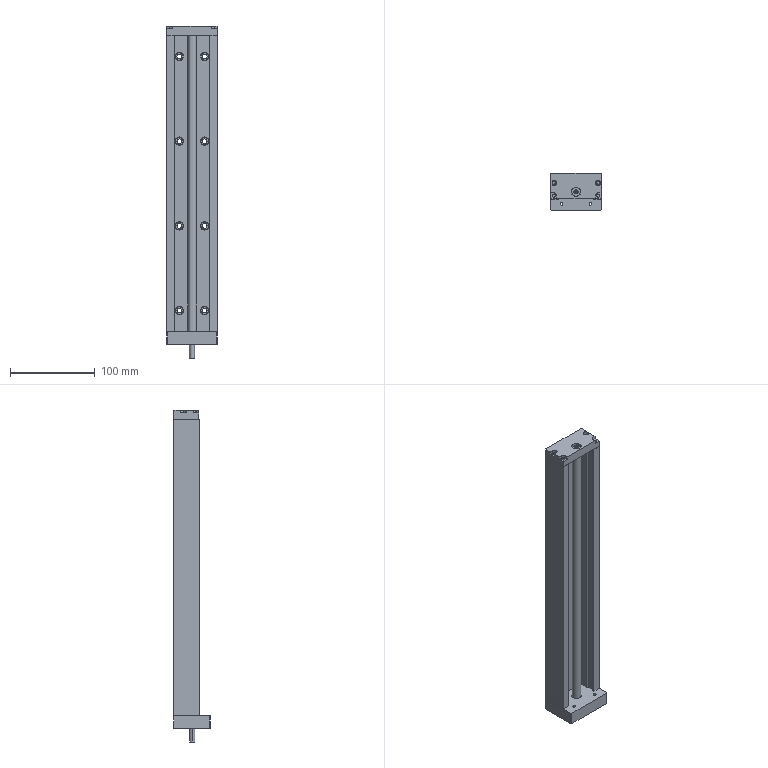Part | SolidWorks | features BaseBody 2 | 2 solids | 145 faces | box 60.2 x 43.4 x 392 mm | volume 378464 mm3 | cylinder 71 | plane 54 | cone 20 | commonest cylinder face diameters 5.5 x16 9 x16 3.242 x8 3.5 x8 6.5 x7 4 x6